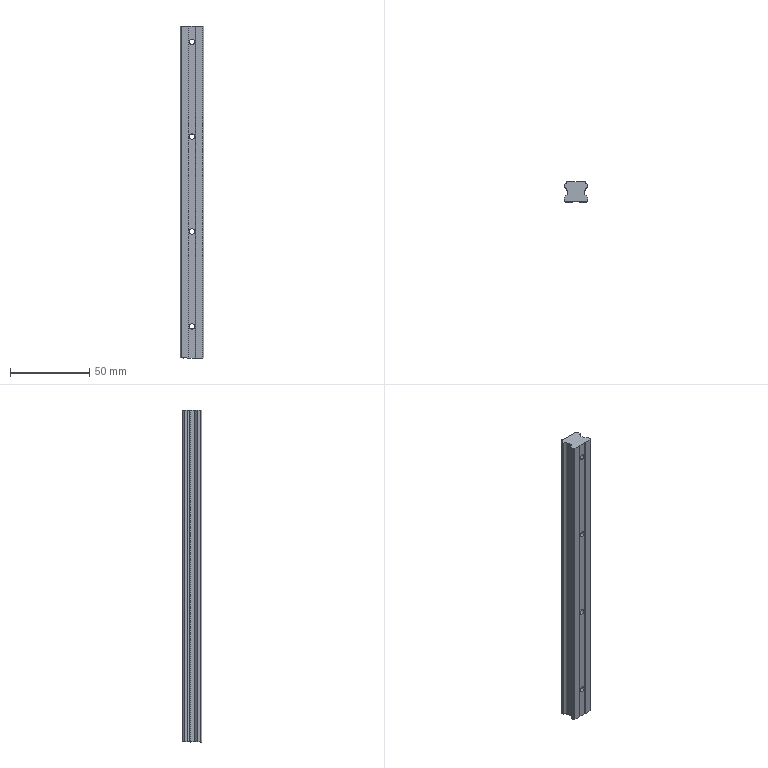Part | SolidWorks | features BaseBody 1, HoleWzd 1, ICE 1, LPattern 1 | 1 solid | 67 faces | box 15 x 12.5 x 210 mm | volume 33443 mm3 | cylinder 40 | plane 27 | commonest cylinder face diameters 0.6 x11 6.5 x8 3.5 x6 6 x6 3 x5 1 x2